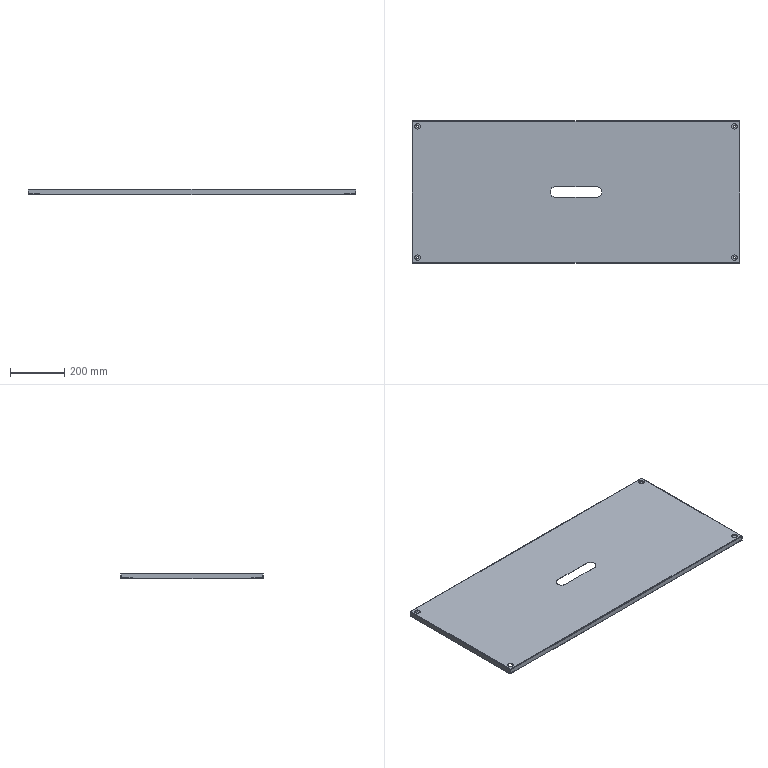Part | STEP file | Box sheet metal 1_default<machined> | 5 solids | 115 faces | box 1203 x 522 x 20 mm | volume 1037743 mm3 | plane 64 | cylinder 31 | spline 20 | commonest cylinder face diameters 7 x8 20 x8 1.5 x4 2 x4 4.5 x4 40 x3